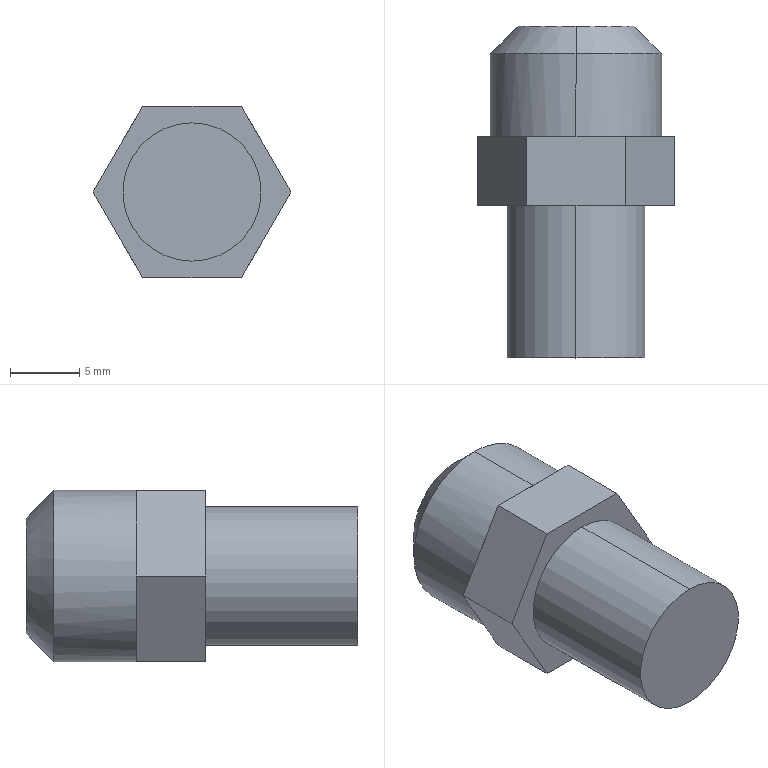Part | SolidWorks | features ICE 2, Chamfer 1, Extrusion 1 | 1 solid | 21 faces | box 14.3 x 24 x 12.384 mm | volume 2422 mm3 | plane 15 | cylinder 4 | cone 2 | commonest cylinder face diameters 10 x2 12.384 x2
STEP:
#1=CARTESIAN_POINT('',(0.,-11.,-5.));
#2=VERTEX_POINT('',#1);
#3=CARTESIAN_POINT('',(0.,-11.,5.));
#4=VERTEX_POINT('',#3);
#5=CARTESIAN_POINT('',(0.,-11.,0.));
#6=DIRECTION('',(0.,-1.,0.));
#7=DIRECTION('',(0.,0.,-1.));
#8=AXIS2_PLACEMENT_3D('',#5,#6,#7);
#9=CIRCLE('',#8,5.);
#10=EDGE_CURVE('',#2,#4,#9,.T.);
#11=ORIENTED_EDGE('',*,*,#10,.F.);
#12=CARTESIAN_POINT('',(0.,0.,-5.));
#13=VERTEX_POINT('',#12);
#14=CARTESIAN_POINT('',(0.,-11.,-5.));
#15=DIRECTION('',(0.,1.,0.));
#16=VECTOR('',#15,1000.);
#17=LINE('',#14,#16);
#18=EDGE_CURVE('',#2,#13,#17,.T.);
#19=ORIENTED_EDGE('',*,*,#18,.T.);
#20=CARTESIAN_POINT('',(0.,0.,5.));
#21=VERTEX_POINT('',#20);
#22=CARTESIAN_POINT('',(0.,0.,0.));
#23=DIRECTION('',(0.,-1.,0.));
#24=DIRECTION('',(0.,0.,1.));
#25=AXIS2_PLACEMENT_3D('',#22,#23,#24);
#26=CIRCLE('',#25,5.);
#27=EDGE_CURVE('',#13,#21,#26,.T.);
#28=ORIENTED_EDGE('',*,*,#27,.T.);
#29=CARTESIAN_POINT('',(0.,-11.,5.));
#30=DIRECTION('',(0.,1.,0.));
#31=VECTOR('',#30,1000.);
#32=LINE('',#29,#31);
#33=EDGE_CURVE('',#4,#21,#32,.T.);
#34=ORIENTED_EDGE('',*,*,#33,.F.);
#35=EDGE_LOOP('',(#11,#19,#28,#34));
#36=FACE_OUTER_BOUND('',#35,.T.);
#37=CARTESIAN_POINT('',(0.,-11.,0.));
#38=DIRECTION('',(0.,1.,0.));
#39=DIRECTION('',(0.,0.,1.));
#40=AXIS2_PLACEMENT_3D('',#37,#38,#39);
#41=CYLINDRICAL_SURFACE('',#40,5.);
#42=ADVANCED_FACE('',(#36),#41,.T.);
#43=CARTESIAN_POINT('',(0.,13.,4.192));
#44=VERTEX_POINT('',#43);
#45=CARTESIAN_POINT('',(0.,13.,-4.192));
#46=VERTEX_POINT('',#45);
#47=CARTESIAN_POINT('',(0.,13.,0.));
#48=DIRECTION('',(0.,1.,0.));
#49=DIRECTION('',(0.,0.,1.));
#50=AXIS2_PLACEMENT_3D('',#47,#48,#49);
#51=CIRCLE('',#50,4.192);
#52=EDGE_CURVE('',#44,#46,#51,.T.);
#53=ORIENTED_EDGE('',*,*,#52,.F.);
#54=CARTESIAN_POINT('',(0.,11.,6.192));
#55=VERTEX_POINT('',#54);
#56=CARTESIAN_POINT('',(0.,13.,4.192));
#57=DIRECTION('',(0.,-0.7071,0.7071));
#58=VECTOR('',#57,1000.);
#59=LINE('',#56,#58);
#60=EDGE_CURVE('',#44,#55,#59,.T.);
#61=ORIENTED_EDGE('',*,*,#60,.T.);
#62=CARTESIAN_POINT('',(0.,11.,-6.192));
#63=VERTEX_POINT('',#62);
#64=CARTESIAN_POINT('',(0.,11.,0.));
#65=DIRECTION('',(0.,-1.,0.));
#66=DIRECTION('',(0.,0.,1.));
#67=AXIS2_PLACEMENT_3D('',#64,#65,#66);
#68=CIRCLE('',#67,6.192);
#69=EDGE_CURVE('',#63,#55,#68,.T.);
#70=ORIENTED_EDGE('',*,*,#69,.F.);
#71=CARTESIAN_POINT('',(0.,13.,-4.192));
#72=DIRECTION('',(0.,-0.7071,-0.7071));
#73=VECTOR('',#72,1000.);
#74=LINE('',#71,#73);
#75=EDGE_CURVE('',#46,#63,#74,.T.);
#76=ORIENTED_EDGE('',*,*,#75,.F.);
#77=EDGE_LOOP('',(#53,#61,#70,#76));
#78=FACE_OUTER_BOUND('',#77,.T.);
#79=CARTESIAN_POINT('',(0.,13.,0.));
#80=DIRECTION('',(0.,-1.,0.));
#81=DIRECTION('',(0.,0.,-1.));
#82=AXIS2_PLACEMENT_3D('',#79,#80,#81);
#83=CONICAL_SURFACE('',#82,4.192,0.7854);
#84=ADVANCED_FACE('',(#78),#83,.T.);
#85=ORIENTED_EDGE('',*,*,#69,.T.);
#86=CARTESIAN_POINT('',(0.,5.,6.192));
#87=VERTEX_POINT('',#86);
#88=CARTESIAN_POINT('',(0.,13.,6.192));
#89=DIRECTION('',(0.,-1.,0.));
#90=VECTOR('',#89,1000.);
#91=LINE('',#88,#90);
#92=EDGE_CURVE('',#55,#87,#91,.T.);
#93=ORIENTED_EDGE('',*,*,#92,.T.);
#94=CARTESIAN_POINT('',(5.363,5.,3.096));
#95=VERTEX_POINT('',#94);
#96=CARTESIAN_POINT('',(0.,5.,0.));
#97=DIRECTION('',(0.,1.,0.));
#98=DIRECTION('',(0.,0.,1.));
#99=AXIS2_PLACEMENT_3D('',#96,#97,#98);
#100=CIRCLE('',#99,6.192);
#101=EDGE_CURVE('',#87,#95,#100,.T.);
#102=ORIENTED_EDGE('',*,*,#101,.T.);
#103=CARTESIAN_POINT('',(5.363,5.,-3.096));
#104=VERTEX_POINT('',#103);
#105=CARTESIAN_POINT('',(0.,5.,0.));
#106=DIRECTION('',(0.,1.,0.));
#107=DIRECTION('',(0.,0.,1.));
#108=AXIS2_PLACEMENT_3D('',#105,#106,#107);
#109=CIRCLE('',#108,6.192);
#110=EDGE_CURVE('',#95,#104,#109,.T.);
#111=ORIENTED_EDGE('',*,*,#110,.T.);
#112=CARTESIAN_POINT('',(0.,5.,-6.192));
#113=VERTEX_POINT('',#112);
#114=CARTESIAN_POINT('',(0.,5.,0.));
#115=DIRECTION('',(0.,1.,0.));
#116=DIRECTION('',(0.,0.,1.));
#117=AXIS2_PLACEMENT_3D('',#114,#115,#116);
#118=CIRCLE('',#117,6.192);
#119=EDGE_CURVE('',#104,#113,#118,.T.);
#120=ORIENTED_EDGE('',*,*,#119,.T.);
#121=CARTESIAN_POINT('',(0.,13.,-6.192));
#122=DIRECTION('',(0.,-1.,0.));
#123=VECTOR('',#122,1000.);
#124=LINE('',#121,#123);
#125=EDGE_CURVE('',#63,#113,#124,.T.);
#126=ORIENTED_EDGE('',*,*,#125,.F.);
#127=EDGE_LOOP('',(#85,#93,#102,#111,#120,#126));
#128=FACE_OUTER_BOUND('',#127,.T.);
#129=CARTESIAN_POINT('',(0.,13.,0.));
#130=DIRECTION('',(0.,-1.,0.));
#131=DIRECTION('',(0.,0.,-1.));
#132=AXIS2_PLACEMENT_3D('',#129,#130,#131);
#133=CYLINDRICAL_SURFACE('',#132,6.192);
#134=ADVANCED_FACE('',(#128),#133,.T.);
#135=CARTESIAN_POINT('',(-3.575,0.,-6.192));
#136=VERTEX_POINT('',#135);
#137=CARTESIAN_POINT('',(-7.15,0.,0.));
#138=VERTEX_POINT('',#137);
#139=CARTESIAN_POINT('',(-3.575,0.,-6.192));
#140=DIRECTION('',(-0.5,0.,0.866));
#141=VECTOR('',#140,1000.);
#142=LINE('',#139,#141);
#143=EDGE_CURVE('',#136,#138,#142,.T.);
#144=ORIENTED_EDGE('',*,*,#143,.F.);
#145=CARTESIAN_POINT('',(3.575,0.,-6.192));
#146=VERTEX_POINT('',#145);
#147=CARTESIAN_POINT('',(3.575,0.,-6.192));
#148=DIRECTION('',(-1.,0.,0.));
#149=VECTOR('',#148,1000.);
#150=LINE('',#147,#149);
#151=EDGE_CURVE('',#146,#136,#150,.T.);
#152=ORIENTED_EDGE('',*,*,#151,.F.);
#153=CARTESIAN_POINT('',(7.15,0.,0.));
#154=VERTEX_POINT('',#153);
#155=CARTESIAN_POINT('',(7.15,0.,0.));
#156=DIRECTION('',(-0.5,0.,-0.866));
#157=VECTOR('',#156,1000.);
#158=LINE('',#155,#157);
#159=EDGE_CURVE('',#154,#146,#158,.T.);
#160=ORIENTED_EDGE('',*,*,#159,.F.);
#161=CARTESIAN_POINT('',(3.575,0.,6.192));
#162=VERTEX_POINT('',#161);
#163=CARTESIAN_POINT('',(3.575,0.,6.192));
#164=DIRECTION('',(0.5,0.,-0.866));
#165=VECTOR('',#164,1000.);
#166=LINE('',#163,#165);
#167=EDGE_CURVE('',#162,#154,#166,.T.);
#168=ORIENTED_EDGE('',*,*,#167,.F.);
#169=CARTESIAN_POINT('',(-3.575,0.,6.192));
#170=VERTEX_POINT('',#169);
#171=CARTESIAN_POINT('',(-3.575,0.,6.192));
#172=DIRECTION('',(1.,0.,0.));
#173=VECTOR('',#172,1000.);
#174=LINE('',#171,#173);
#175=EDGE_CURVE('',#170,#162,#174,.T.);
#176=ORIENTED_EDGE('',*,*,#175,.F.);
#177=CARTESIAN_POINT('',(-7.15,0.,0.));
#178=DIRECTION('',(0.5,0.,0.866));
#179=VECTOR('',#178,1000.);
#180=LINE('',#177,#179);
#181=EDGE_CURVE('',#138,#170,#180,.T.);
#182=ORIENTED_EDGE('',*,*,#181,.F.);
#183=EDGE_LOOP('',(#144,#152,#160,#168,#176,#182));
#184=FACE_OUTER_BOUND('',#183,.T.);
#185=CARTESIAN_POINT('',(0.,0.,0.));
#186=DIRECTION('',(0.,-1.,0.));
#187=DIRECTION('',(0.,0.,1.));
#188=AXIS2_PLACEMENT_3D('',#185,#186,#187);
#189=CIRCLE('',#188,5.);
#190=EDGE_CURVE('',#21,#13,#189,.T.);
#191=ORIENTED_EDGE('',*,*,#190,.F.);
#192=ORIENTED_EDGE('',*,*,#27,.F.);
#193=EDGE_LOOP('',(#191,#192));
#194=FACE_BOUND('',#193,.T.);
#195=CARTESIAN_POINT('',(0.,0.,0.));
#196=DIRECTION('',(0.,1.,0.));
#197=DIRECTION('',(0.,0.,1.));
#198=AXIS2_PLACEMENT_3D('',#195,#196,#197);
#199=PLANE('',#198);
#200=ADVANCED_FACE('',(#184,#194),#199,.F.);
#201=ORIENTED_EDGE('',*,*,#101,.F.);
#202=CARTESIAN_POINT('',(3.575,5.,6.192));
#203=VERTEX_POINT('',#202);
#204=CARTESIAN_POINT('',(-3.575,5.,6.192));
#205=DIRECTION('',(1.,0.,0.));
#206=VECTOR('',#205,1000.);
#207=LINE('',#204,#206);
#208=EDGE_CURVE('',#87,#203,#207,.T.);
#209=ORIENTED_EDGE('',*,*,#208,.T.);
#210=CARTESIAN_POINT('',(3.575,5.,6.192));
#211=DIRECTION('',(0.5,0.,-0.866));
#212=VECTOR('',#211,1000.);
#213=LINE('',#210,#212);
#214=EDGE_CURVE('',#203,#95,#213,.T.);
#215=ORIENTED_EDGE('',*,*,#214,.T.);
#216=EDGE_LOOP('',(#201,#209,#215));
#217=FACE_OUTER_BOUND('',#216,.T.);
#218=CARTESIAN_POINT('',(0.,5.,0.));
#219=DIRECTION('',(0.,1.,0.));
#220=DIRECTION('',(0.,0.,1.));
#221=AXIS2_PLACEMENT_3D('',#218,#219,#220);
#222=PLANE('',#221);
#223=ADVANCED_FACE('',(#217),#222,.T.);
#224=ORIENTED_EDGE('',*,*,#110,.F.);
#225=CARTESIAN_POINT('',(7.15,5.,0.));
#226=VERTEX_POINT('',#225);
#227=CARTESIAN_POINT('',(3.575,5.,6.192));
#228=DIRECTION('',(0.5,0.,-0.866));
#229=VECTOR('',#228,1000.);
#230=LINE('',#227,#229);
#231=EDGE_CURVE('',#95,#226,#230,.T.);
#232=ORIENTED_EDGE('',*,*,#231,.T.);
#233=CARTESIAN_POINT('',(7.15,5.,0.));
#234=DIRECTION('',(-0.5,0.,-0.866));
#235=VECTOR('',#234,1000.);
#236=LINE('',#233,#235);
#237=EDGE_CURVE('',#226,#104,#236,.T.);
#238=ORIENTED_EDGE('',*,*,#237,.T.);
#239=EDGE_LOOP('',(#224,#232,#238));
#240=FACE_OUTER_BOUND('',#239,.T.);
#241=CARTESIAN_POINT('',(0.,5.,0.));
#242=DIRECTION('',(0.,1.,0.));
#243=DIRECTION('',(0.,0.,1.));
#244=AXIS2_PLACEMENT_3D('',#241,#242,#243);
#245=PLANE('',#244);
#246=ADVANCED_FACE('',(#240),#245,.T.);
#247=ORIENTED_EDGE('',*,*,#119,.F.);
#248=CARTESIAN_POINT('',(3.575,5.,-6.192));
#249=VERTEX_POINT('',#248);
#250=CARTESIAN_POINT('',(7.15,5.,0.));
#251=DIRECTION('',(-0.5,0.,-0.866));
#252=VECTOR('',#251,1000.);
#253=LINE('',#250,#252);
#254=EDGE_CURVE('',#104,#249,#253,.T.);
#255=ORIENTED_EDGE('',*,*,#254,.T.);
#256=CARTESIAN_POINT('',(3.575,5.,-6.192));
#257=DIRECTION('',(-1.,0.,0.));
#258=VECTOR('',#257,1000.);
#259=LINE('',#256,#258);
#260=EDGE_CURVE('',#249,#113,#259,.T.);
#261=ORIENTED_EDGE('',*,*,#260,.T.);
#262=EDGE_LOOP('',(#247,#255,#261));
#263=FACE_OUTER_BOUND('',#262,.T.);
#264=CARTESIAN_POINT('',(0.,5.,0.));
#265=DIRECTION('',(0.,1.,0.));
#266=DIRECTION('',(0.,0.,1.));
#267=AXIS2_PLACEMENT_3D('',#264,#265,#266);
#268=PLANE('',#267);
#269=ADVANCED_FACE('',(#263),#268,.T.);
#270=CARTESIAN_POINT('',(-5.362,5.,-3.096));
#271=VERTEX_POINT('',#270);
#272=CARTESIAN_POINT('',(0.,5.,0.));
#273=DIRECTION('',(0.,1.,0.));
#274=DIRECTION('',(0.,0.,1.));
#275=AXIS2_PLACEMENT_3D('',#272,#273,#274);
#276=CIRCLE('',#275,6.192);
#277=EDGE_CURVE('',#113,#271,#276,.T.);
#278=ORIENTED_EDGE('',*,*,#277,.F.);
#279=CARTESIAN_POINT('',(-3.575,5.,-6.192));
#280=VERTEX_POINT('',#279);
#281=CARTESIAN_POINT('',(3.575,5.,-6.192));
#282=DIRECTION('',(-1.,0.,0.));
#283=VECTOR('',#282,1000.);
#284=LINE('',#281,#283);
#285=EDGE_CURVE('',#113,#280,#284,.T.);
#286=ORIENTED_EDGE('',*,*,#285,.T.);
#287=CARTESIAN_POINT('',(-3.575,5.,-6.192));
#288=DIRECTION('',(-0.5,0.,0.866));
#289=VECTOR('',#288,1000.);
#290=LINE('',#287,#289);
#291=EDGE_CURVE('',#280,#271,#290,.T.);
#292=ORIENTED_EDGE('',*,*,#291,.T.);
#293=EDGE_LOOP('',(#278,#286,#292));
#294=FACE_OUTER_BOUND('',#293,.T.);
#295=CARTESIAN_POINT('',(0.,5.,0.));
#296=DIRECTION('',(0.,1.,0.));
#297=DIRECTION('',(0.,0.,1.));
#298=AXIS2_PLACEMENT_3D('',#295,#296,#297);
#299=PLANE('',#298);
#300=ADVANCED_FACE('',(#294),#299,.T.);
#301=CARTESIAN_POINT('',(-5.362,5.,3.096));
#302=VERTEX_POINT('',#301);
#303=CARTESIAN_POINT('',(0.,5.,0.));
#304=DIRECTION('',(0.,1.,0.));
#305=DIRECTION('',(0.,0.,1.));
#306=AXIS2_PLACEMENT_3D('',#303,#304,#305);
#307=CIRCLE('',#306,6.192);
#308=EDGE_CURVE('',#271,#302,#307,.T.);
#309=ORIENTED_EDGE('',*,*,#308,.F.);
#310=CARTESIAN_POINT('',(-7.15,5.,0.));
#311=VERTEX_POINT('',#310);
#312=CARTESIAN_POINT('',(-3.575,5.,-6.192));
#313=DIRECTION('',(-0.5,0.,0.866));
#314=VECTOR('',#313,1000.);
#315=LINE('',#312,#314);
#316=EDGE_CURVE('',#271,#311,#315,.T.);
#317=ORIENTED_EDGE('',*,*,#316,.T.);
#318=CARTESIAN_POINT('',(-7.15,5.,0.));
#319=DIRECTION('',(0.5,0.,0.866));
#320=VECTOR('',#319,1000.);
#321=LINE('',#318,#320);
#322=EDGE_CURVE('',#311,#302,#321,.T.);
#323=ORIENTED_EDGE('',*,*,#322,.T.);
#324=EDGE_LOOP('',(#309,#317,#323));
#325=FACE_OUTER_BOUND('',#324,.T.);
#326=CARTESIAN_POINT('',(0.,5.,0.));
#327=DIRECTION('',(0.,1.,0.));
#328=DIRECTION('',(0.,0.,1.));
#329=AXIS2_PLACEMENT_3D('',#326,#327,#328);
#330=PLANE('',#329);
#331=ADVANCED_FACE('',(#325),#330,.T.);
#332=ORIENTED_EDGE('',*,*,#143,.T.);
#333=CARTESIAN_POINT('',(-7.15,5.,0.));
#334=DIRECTION('',(0.,-1.,0.));
#335=VECTOR('',#334,1000.);
#336=LINE('',#333,#335);
#337=EDGE_CURVE('',#311,#138,#336,.T.);
#338=ORIENTED_EDGE('',*,*,#337,.F.);
#339=ORIENTED_EDGE('',*,*,#316,.F.);
#340=ORIENTED_EDGE('',*,*,#291,.F.);
#341=CARTESIAN_POINT('',(-3.575,5.,-6.192));
#342=DIRECTION('',(0.,-1.,0.));
#343=VECTOR('',#342,1000.);
#344=LINE('',#341,#343);
#345=EDGE_CURVE('',#280,#136,#344,.T.);
#346=ORIENTED_EDGE('',*,*,#345,.T.);
#347=EDGE_LOOP('',(#332,#338,#339,#340,#346));
#348=FACE_OUTER_BOUND('',#347,.T.);
#349=CARTESIAN_POINT('',(-3.575,5.,-6.192));
#350=DIRECTION('',(0.866,0.,0.5));
#351=DIRECTION('',(0.5,0.,-0.866));
#352=AXIS2_PLACEMENT_3D('',#349,#350,#351);
#353=PLANE('',#352);
#354=ADVANCED_FACE('',(#348),#353,.F.);
#355=ORIENTED_EDGE('',*,*,#181,.T.);
#356=CARTESIAN_POINT('',(-3.575,5.,6.192));
#357=VERTEX_POINT('',#356);
#358=CARTESIAN_POINT('',(-3.575,5.,6.192));
#359=DIRECTION('',(0.,-1.,0.));
#360=VECTOR('',#359,1000.);
#361=LINE('',#358,#360);
#362=EDGE_CURVE('',#357,#170,#361,.T.);
#363=ORIENTED_EDGE('',*,*,#362,.F.);
#364=CARTESIAN_POINT('',(-7.15,5.,0.));
#365=DIRECTION('',(0.5,0.,0.866));
#366=VECTOR('',#365,1000.);
#367=LINE('',#364,#366);
#368=EDGE_CURVE('',#302,#357,#367,.T.);
#369=ORIENTED_EDGE('',*,*,#368,.F.);
#370=ORIENTED_EDGE('',*,*,#322,.F.);
#371=ORIENTED_EDGE('',*,*,#337,.T.);
#372=EDGE_LOOP('',(#355,#363,#369,#370,#371));
#373=FACE_OUTER_BOUND('',#372,.T.);
#374=CARTESIAN_POINT('',(-7.15,5.,0.));
#375=DIRECTION('',(0.866,0.,-0.5));
#376=DIRECTION('',(-0.5,0.,-0.866));
#377=AXIS2_PLACEMENT_3D('',#374,#375,#376);
#378=PLANE('',#377);
#379=ADVANCED_FACE('',(#373),#378,.F.);
#380=ORIENTED_EDGE('',*,*,#175,.T.);
#381=CARTESIAN_POINT('',(3.575,5.,6.192));
#382=DIRECTION('',(0.,-1.,0.));
#383=VECTOR('',#382,1000.);
#384=LINE('',#381,#383);
#385=EDGE_CURVE('',#203,#162,#384,.T.);
#386=ORIENTED_EDGE('',*,*,#385,.F.);
#387=ORIENTED_EDGE('',*,*,#208,.F.);
#388=CARTESIAN_POINT('',(-3.575,5.,6.192));
#389=DIRECTION('',(1.,0.,0.));
#390=VECTOR('',#389,1000.);
#391=LINE('',#388,#390);
#392=EDGE_CURVE('',#357,#87,#391,.T.);
#393=ORIENTED_EDGE('',*,*,#392,.F.);
#394=ORIENTED_EDGE('',*,*,#362,.T.);
#395=EDGE_LOOP('',(#380,#386,#387,#393,#394));
#396=FACE_OUTER_BOUND('',#395,.T.);
#397=CARTESIAN_POINT('',(-3.575,5.,6.192));
#398=DIRECTION('',(0.,0.,-1.));
#399=DIRECTION('',(-1.,0.,0.));
#400=AXIS2_PLACEMENT_3D('',#397,#398,#399);
#401=PLANE('',#400);
#402=ADVANCED_FACE('',(#396),#401,.F.);
#403=ORIENTED_EDGE('',*,*,#167,.T.);
#404=CARTESIAN_POINT('',(7.15,5.,0.));
#405=DIRECTION('',(0.,-1.,0.));
#406=VECTOR('',#405,1000.);
#407=LINE('',#404,#406);
#408=EDGE_CURVE('',#226,#154,#407,.T.);
#409=ORIENTED_EDGE('',*,*,#408,.F.);
#410=ORIENTED_EDGE('',*,*,#231,.F.);
#411=ORIENTED_EDGE('',*,*,#214,.F.);
#412=ORIENTED_EDGE('',*,*,#385,.T.);
#413=EDGE_LOOP('',(#403,#409,#410,#411,#412));
#414=FACE_OUTER_BOUND('',#413,.T.);
#415=CARTESIAN_POINT('',(3.575,5.,6.192));
#416=DIRECTION('',(-0.866,0.,-0.5));
#417=DIRECTION('',(-0.5,0.,0.866));
#418=AXIS2_PLACEMENT_3D('',#415,#416,#417);
#419=PLANE('',#418);
#420=ADVANCED_FACE('',(#414),#419,.F.);
#421=ORIENTED_EDGE('',*,*,#159,.T.);
#422=CARTESIAN_POINT('',(3.575,5.,-6.192));
#423=DIRECTION('',(0.,-1.,0.));
#424=VECTOR('',#423,1000.);
#425=LINE('',#422,#424);
#426=EDGE_CURVE('',#249,#146,#425,.T.);
#427=ORIENTED_EDGE('',*,*,#426,.F.);
#428=ORIENTED_EDGE('',*,*,#254,.F.);
#429=ORIENTED_EDGE('',*,*,#237,.F.);
#430=ORIENTED_EDGE('',*,*,#408,.T.);
#431=EDGE_LOOP('',(#421,#427,#428,#429,#430));
#432=FACE_OUTER_BOUND('',#431,.T.);
#433=CARTESIAN_POINT('',(7.15,5.,0.));
#434=DIRECTION('',(-0.866,0.,0.5));
#435=DIRECTION('',(0.5,0.,0.866));
#436=AXIS2_PLACEMENT_3D('',#433,#434,#435);
#437=PLANE('',#436);
#438=ADVANCED_FACE('',(#432),#437,.F.);
#439=ORIENTED_EDGE('',*,*,#151,.T.);
#440=ORIENTED_EDGE('',*,*,#345,.F.);
#441=ORIENTED_EDGE('',*,*,#285,.F.);
#442=ORIENTED_EDGE('',*,*,#260,.F.);
#443=ORIENTED_EDGE('',*,*,#426,.T.);
#444=EDGE_LOOP('',(#439,#440,#441,#442,#443));
#445=FACE_OUTER_BOUND('',#444,.T.);
#446=CARTESIAN_POINT('',(3.575,5.,-6.192));
#447=DIRECTION('',(0.,0.,1.));
#448=DIRECTION('',(1.,0.,0.));
#449=AXIS2_PLACEMENT_3D('',#446,#447,#448);
#450=PLANE('',#449);
#451=ADVANCED_FACE('',(#445),#450,.F.);
#452=CARTESIAN_POINT('',(0.,5.,0.));
#453=DIRECTION('',(0.,1.,0.));
#454=DIRECTION('',(0.,0.,1.));
#455=AXIS2_PLACEMENT_3D('',#452,#453,#454);
#456=CIRCLE('',#455,6.192);
#457=EDGE_CURVE('',#302,#87,#456,.T.);
#458=ORIENTED_EDGE('',*,*,#457,.F.);
#459=ORIENTED_EDGE('',*,*,#368,.T.);
#460=ORIENTED_EDGE('',*,*,#392,.T.);
#461=EDGE_LOOP('',(#458,#459,#460));
#462=FACE_OUTER_BOUND('',#461,.T.);
#463=CARTESIAN_POINT('',(0.,5.,0.));
#464=DIRECTION('',(0.,1.,0.));
#465=DIRECTION('',(0.,0.,1.));
#466=AXIS2_PLACEMENT_3D('',#463,#464,#465);
#467=PLANE('',#466);
#468=ADVANCED_FACE('',(#462),#467,.T.);
#469=ORIENTED_EDGE('',*,*,#92,.F.);
#470=CARTESIAN_POINT('',(0.,11.,0.));
#471=DIRECTION('',(0.,-1.,0.));
#472=DIRECTION('',(0.,0.,1.));
#473=AXIS2_PLACEMENT_3D('',#470,#471,#472);
#474=CIRCLE('',#473,6.192);
#475=EDGE_CURVE('',#55,#63,#474,.T.);
#476=ORIENTED_EDGE('',*,*,#475,.T.);
#477=ORIENTED_EDGE('',*,*,#125,.T.);
#478=ORIENTED_EDGE('',*,*,#277,.T.);
#479=ORIENTED_EDGE('',*,*,#308,.T.);
#480=ORIENTED_EDGE('',*,*,#457,.T.);
#481=EDGE_LOOP('',(#469,#476,#477,#478,#479,#480));
#482=FACE_OUTER_BOUND('',#481,.T.);
#483=CARTESIAN_POINT('',(0.,13.,0.));
#484=DIRECTION('',(0.,-1.,0.));
#485=DIRECTION('',(0.,0.,-1.));
#486=AXIS2_PLACEMENT_3D('',#483,#484,#485);
#487=CYLINDRICAL_SURFACE('',#486,6.192);
#488=ADVANCED_FACE('',(#482),#487,.T.);
#489=CARTESIAN_POINT('',(0.,13.,0.));
#490=DIRECTION('',(0.,1.,0.));
#491=DIRECTION('',(0.,0.,1.));
#492=AXIS2_PLACEMENT_3D('',#489,#490,#491);
#493=CIRCLE('',#492,4.192);
#494=EDGE_CURVE('',#46,#44,#493,.T.);
#495=ORIENTED_EDGE('',*,*,#494,.T.);
#496=ORIENTED_EDGE('',*,*,#52,.T.);
#497=EDGE_LOOP('',(#495,#496));
#498=FACE_OUTER_BOUND('',#497,.T.);
#499=CARTESIAN_POINT('',(0.,13.,0.));
#500=DIRECTION('',(0.,1.,0.));
#501=DIRECTION('',(0.,0.,1.));
#502=AXIS2_PLACEMENT_3D('',#499,#500,#501);
#503=PLANE('',#502);
#504=ADVANCED_FACE('',(#498),#503,.T.);
#505=ORIENTED_EDGE('',*,*,#60,.F.);
#506=ORIENTED_EDGE('',*,*,#494,.F.);
#507=ORIENTED_EDGE('',*,*,#75,.T.);
#508=ORIENTED_EDGE('',*,*,#475,.F.);
#509=EDGE_LOOP('',(#505,#506,#507,#508));
#510=FACE_OUTER_BOUND('',#509,.T.);
#511=CARTESIAN_POINT('',(0.,13.,0.));
#512=DIRECTION('',(0.,-1.,0.));
#513=DIRECTION('',(0.,0.,-1.));
#514=AXIS2_PLACEMENT_3D('',#511,#512,#513);
#515=CONICAL_SURFACE('',#514,4.192,0.7854);
#516=ADVANCED_FACE('',(#510),#515,.T.);
#517=ORIENTED_EDGE('',*,*,#18,.F.);
#518=CARTESIAN_POINT('',(0.,-11.,0.));
#519=DIRECTION('',(0.,-1.,0.));
#520=DIRECTION('',(0.,0.,-1.));
#521=AXIS2_PLACEMENT_3D('',#518,#519,#520);
#522=CIRCLE('',#521,5.);
#523=EDGE_CURVE('',#4,#2,#522,.T.);
#524=ORIENTED_EDGE('',*,*,#523,.F.);
#525=ORIENTED_EDGE('',*,*,#33,.T.);
#526=ORIENTED_EDGE('',*,*,#190,.T.);
#527=EDGE_LOOP('',(#517,#524,#525,#526));
#528=FACE_OUTER_BOUND('',#527,.T.);
#529=CARTESIAN_POINT('',(0.,-11.,0.));
#530=DIRECTION('',(0.,1.,0.));
#531=DIRECTION('',(0.,0.,1.));
#532=AXIS2_PLACEMENT_3D('',#529,#530,#531);
#533=CYLINDRICAL_SURFACE('',#532,5.);
#534=ADVANCED_FACE('',(#528),#533,.T.);
#535=ORIENTED_EDGE('',*,*,#523,.T.);
#536=ORIENTED_EDGE('',*,*,#10,.T.);
#537=EDGE_LOOP('',(#535,#536));
#538=FACE_OUTER_BOUND('',#537,.T.);
#539=CARTESIAN_POINT('',(0.,-11.,0.));
#540=DIRECTION('',(0.,-1.,0.));
#541=DIRECTION('',(0.,0.,-1.));
#542=AXIS2_PLACEMENT_3D('',#539,#540,#541);
#543=PLANE('',#542);
#544=ADVANCED_FACE('',(#538),#543,.T.);
#545=CLOSED_SHELL('',(#42,#84,#134,#200,#223,#246,#269,#300,#331,#354,#379,#402,#420,#438,#451,#468,#488,#504,#516,#534,#544));
#546=MANIFOLD_SOLID_BREP('',#545);
#547=CARTESIAN_POINT('',(0.,0.,0.));
#548=DIRECTION('',(0.,0.,1.));
#549=DIRECTION('',(1.,0.,0.));
#550=AXIS2_PLACEMENT_3D('',#547,#548,#549);
#551=(LENGTH_UNIT()NAMED_UNIT(*)SI_UNIT(.MILLI.,.METRE.));
#552=UNCERTAINTY_MEASURE_WITH_UNIT(LENGTH_MEASURE(0.00001),#551,'','');
#553=(NAMED_UNIT(*)PLANE_ANGLE_UNIT()SI_UNIT($,.RADIAN.));
#554=(NAMED_UNIT(*)SI_UNIT($,.STERADIAN.)SOLID_ANGLE_UNIT());
#555=(GEOMETRIC_REPRESENTATION_CONTEXT(3)GLOBAL_UNCERTAINTY_ASSIGNED_CONTEXT((#552))GLOBAL_UNIT_ASSIGNED_CONTEXT((#551,#553,#554))REPRESENTATION_CONTEXT('',''));
#556=ADVANCED_BREP_SHAPE_REPRESENTATION('',(#546,#550),#555);